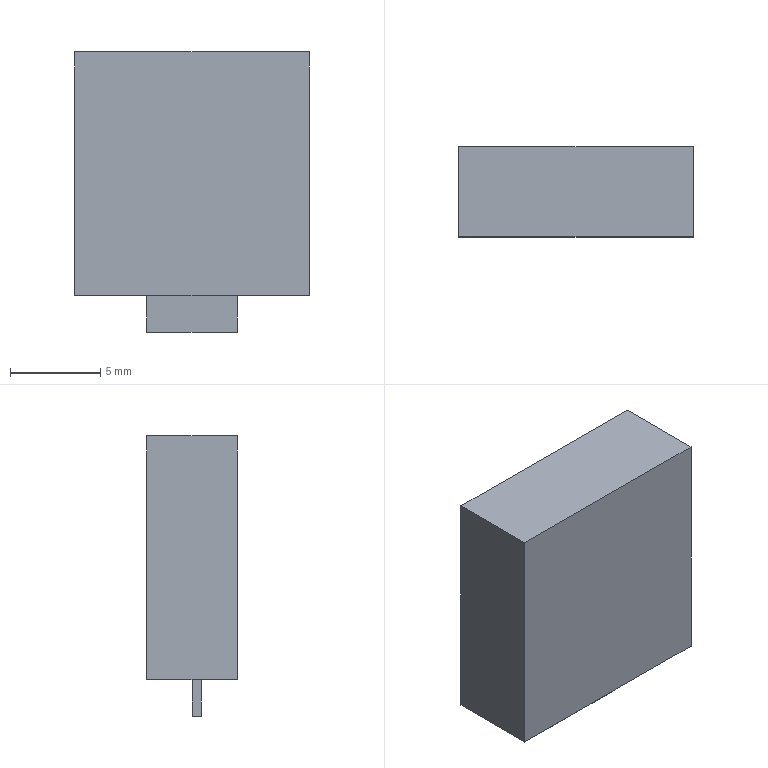Part | STEP file | 0245_028_FPCN14 | 1 solid | 11 faces | box 13 x 5 x 15.5 mm | volume 882.5 mm3 | plane 11
STEP:
#1=CARTESIAN_POINT('',(0.,0.,0.));
#2=DIRECTION('',(0.,0.,1.));
#3=DIRECTION('',(1.,0.,0.));
#4=AXIS2_PLACEMENT_3D('',#1,#2,#3);
#5=CARTESIAN_POINT('',(-6.5,5.,0.));
#6=VERTEX_POINT('',#5);
#7=CARTESIAN_POINT('',(-6.5,0.,0.));
#8=VERTEX_POINT('',#7);
#9=CARTESIAN_POINT('',(-6.5,0.,0.));
#10=DIRECTION('',(0.,-1.,0.));
#11=VECTOR('',#10,1.);
#12=LINE('',#9,#11);
#13=CARTESIAN_POINT('',(-6.5,5.,0.));
#14=DIRECTION('',(0.,0.,-1.));
#15=DIRECTION('',(-1.,0.,0.));
#16=AXIS2_PLACEMENT_3D('',#13,#14,#15);
#17=PLANE('',#16);
#18=CARTESIAN_POINT('',(0.,-5.));
#19=DIRECTION('',(0.,-1.));
#20=VECTOR('',#19,1.);
#21=LINE('',#18,#20);
#22=(GEOMETRIC_REPRESENTATION_CONTEXT(2)PARAMETRIC_REPRESENTATION_CONTEXT()REPRESENTATION_CONTEXT('',''));
#23=DEFINITIONAL_REPRESENTATION('',(#21),#22);
#24=PCURVE('',#17,#23);
#25=CARTESIAN_POINT('',(-6.5,0.,13.5));
#26=DIRECTION('',(1.,0.,0.));
#27=DIRECTION('',(0.,1.,0.));
#28=AXIS2_PLACEMENT_3D('',#25,#26,#27);
#29=PLANE('',#28);
#30=CARTESIAN_POINT('',(0.,-13.5));
#31=DIRECTION('',(-1.,0.));
#32=VECTOR('',#31,1.);
#33=LINE('',#30,#32);
#34=(GEOMETRIC_REPRESENTATION_CONTEXT(2)PARAMETRIC_REPRESENTATION_CONTEXT()REPRESENTATION_CONTEXT('',''));
#35=DEFINITIONAL_REPRESENTATION('',(#33),#34);
#36=PCURVE('',#29,#35);
#37=SURFACE_CURVE('',#12,(#24,#36),.PCURVE_S1.);
#38=EDGE_CURVE('',#6,#8,#37,.T.);
#39=ORIENTED_EDGE('',*,*,#38,.F.);
#40=CARTESIAN_POINT('',(6.5,5.,0.));
#41=VERTEX_POINT('',#40);
#42=CARTESIAN_POINT('',(-6.5,5.,0.));
#43=DIRECTION('',(-1.,0.,0.));
#44=VECTOR('',#43,1.);
#45=LINE('',#42,#44);
#46=CARTESIAN_POINT('',(0.,0.));
#47=DIRECTION('',(1.,0.));
#48=VECTOR('',#47,1.);
#49=LINE('',#46,#48);
#50=(GEOMETRIC_REPRESENTATION_CONTEXT(2)PARAMETRIC_REPRESENTATION_CONTEXT()REPRESENTATION_CONTEXT('',''));
#51=DEFINITIONAL_REPRESENTATION('',(#49),#50);
#52=PCURVE('',#17,#51);
#53=CARTESIAN_POINT('',(-6.5,5.,13.5));
#54=DIRECTION('',(0.,-1.,0.));
#55=DIRECTION('',(0.,0.,-1.));
#56=AXIS2_PLACEMENT_3D('',#53,#54,#55);
#57=PLANE('',#56);
#58=CARTESIAN_POINT('',(13.5,0.));
#59=DIRECTION('',(0.,-1.));
#60=VECTOR('',#59,1.);
#61=LINE('',#58,#60);
#62=(GEOMETRIC_REPRESENTATION_CONTEXT(2)PARAMETRIC_REPRESENTATION_CONTEXT()REPRESENTATION_CONTEXT('',''));
#63=DEFINITIONAL_REPRESENTATION('',(#61),#62);
#64=PCURVE('',#57,#63);
#65=SURFACE_CURVE('',#45,(#52,#64),.PCURVE_S1.);
#66=EDGE_CURVE('',#41,#6,#65,.T.);
#67=ORIENTED_EDGE('',*,*,#66,.F.);
#68=CARTESIAN_POINT('',(6.5,0.,0.));
#69=VERTEX_POINT('',#68);
#70=CARTESIAN_POINT('',(6.5,0.,0.));
#71=DIRECTION('',(0.,1.,0.));
#72=VECTOR('',#71,1.);
#73=LINE('',#70,#72);
#74=CARTESIAN_POINT('',(-13.,-5.));
#75=DIRECTION('',(0.,1.));
#76=VECTOR('',#75,1.);
#77=LINE('',#74,#76);
#78=(GEOMETRIC_REPRESENTATION_CONTEXT(2)PARAMETRIC_REPRESENTATION_CONTEXT()REPRESENTATION_CONTEXT('',''));
#79=DEFINITIONAL_REPRESENTATION('',(#77),#78);
#80=PCURVE('',#17,#79);
#81=CARTESIAN_POINT('',(6.5,0.,13.5));
#82=DIRECTION('',(-1.,0.,0.));
#83=DIRECTION('',(0.,-1.,0.));
#84=AXIS2_PLACEMENT_3D('',#81,#82,#83);
#85=PLANE('',#84);
#86=CARTESIAN_POINT('',(0.,-13.5));
#87=DIRECTION('',(-1.,0.));
#88=VECTOR('',#87,1.);
#89=LINE('',#86,#88);
#90=(GEOMETRIC_REPRESENTATION_CONTEXT(2)PARAMETRIC_REPRESENTATION_CONTEXT()REPRESENTATION_CONTEXT('',''));
#91=DEFINITIONAL_REPRESENTATION('',(#89),#90);
#92=PCURVE('',#85,#91);
#93=SURFACE_CURVE('',#73,(#80,#92),.PCURVE_S1.);
#94=EDGE_CURVE('',#69,#41,#93,.T.);
#95=ORIENTED_EDGE('',*,*,#94,.F.);
#96=CARTESIAN_POINT('',(-6.5,0.,0.));
#97=DIRECTION('',(1.,0.,0.));
#98=VECTOR('',#97,1.);
#99=LINE('',#96,#98);
#100=CARTESIAN_POINT('',(0.,-5.));
#101=DIRECTION('',(-1.,0.));
#102=VECTOR('',#101,1.);
#103=LINE('',#100,#102);
#104=(GEOMETRIC_REPRESENTATION_CONTEXT(2)PARAMETRIC_REPRESENTATION_CONTEXT()REPRESENTATION_CONTEXT('',''));
#105=DEFINITIONAL_REPRESENTATION('',(#103),#104);
#106=PCURVE('',#17,#105);
#107=CARTESIAN_POINT('',(-6.5,0.,13.5));
#108=DIRECTION('',(0.,1.,0.));
#109=DIRECTION('',(-1.,0.,0.));
#110=AXIS2_PLACEMENT_3D('',#107,#108,#109);
#111=PLANE('',#110);
#112=CARTESIAN_POINT('',(0.,-13.5));
#113=DIRECTION('',(-1.,0.));
#114=VECTOR('',#113,1.);
#115=LINE('',#112,#114);
#116=(GEOMETRIC_REPRESENTATION_CONTEXT(2)PARAMETRIC_REPRESENTATION_CONTEXT()REPRESENTATION_CONTEXT('',''));
#117=DEFINITIONAL_REPRESENTATION('',(#115),#116);
#118=PCURVE('',#111,#117);
#119=SURFACE_CURVE('',#99,(#106,#118),.PCURVE_S1.);
#120=EDGE_CURVE('',#8,#69,#119,.T.);
#121=ORIENTED_EDGE('',*,*,#120,.F.);
#122=EDGE_LOOP('',(#39,#67,#95,#121));
#123=FACE_BOUND('',#122,.T.);
#124=CARTESIAN_POINT('',(2.5,2.,0.));
#125=VERTEX_POINT('',#124);
#126=CARTESIAN_POINT('',(-2.5,2.,0.));
#127=VERTEX_POINT('',#126);
#128=CARTESIAN_POINT('',(2.5,2.,0.));
#129=DIRECTION('',(-1.,0.,0.));
#130=VECTOR('',#129,1.);
#131=LINE('',#128,#130);
#132=CARTESIAN_POINT('',(-9.,-3.));
#133=DIRECTION('',(1.,0.));
#134=VECTOR('',#133,1.);
#135=LINE('',#132,#134);
#136=(GEOMETRIC_REPRESENTATION_CONTEXT(2)PARAMETRIC_REPRESENTATION_CONTEXT()REPRESENTATION_CONTEXT('',''));
#137=DEFINITIONAL_REPRESENTATION('',(#135),#136);
#138=PCURVE('',#17,#137);
#139=CARTESIAN_POINT('',(2.5,2.,-2.));
#140=DIRECTION('',(0.,1.,0.));
#141=DIRECTION('',(0.,0.,1.));
#142=AXIS2_PLACEMENT_3D('',#139,#140,#141);
#143=PLANE('',#142);
#144=CARTESIAN_POINT('',(2.,0.));
#145=DIRECTION('',(0.,-1.));
#146=VECTOR('',#145,1.);
#147=LINE('',#144,#146);
#148=(GEOMETRIC_REPRESENTATION_CONTEXT(2)PARAMETRIC_REPRESENTATION_CONTEXT()REPRESENTATION_CONTEXT('',''));
#149=DEFINITIONAL_REPRESENTATION('',(#147),#148);
#150=PCURVE('',#143,#149);
#151=SURFACE_CURVE('',#131,(#138,#150),.PCURVE_S1.);
#152=EDGE_CURVE('',#125,#127,#151,.T.);
#153=ORIENTED_EDGE('',*,*,#152,.F.);
#154=CARTESIAN_POINT('',(2.5,2.5,0.));
#155=VERTEX_POINT('',#154);
#156=CARTESIAN_POINT('',(2.5,2.5,0.));
#157=DIRECTION('',(0.,-1.,0.));
#158=VECTOR('',#157,1.);
#159=LINE('',#156,#158);
#160=CARTESIAN_POINT('',(-9.,-2.5));
#161=DIRECTION('',(0.,-1.));
#162=VECTOR('',#161,1.);
#163=LINE('',#160,#162);
#164=(GEOMETRIC_REPRESENTATION_CONTEXT(2)PARAMETRIC_REPRESENTATION_CONTEXT()REPRESENTATION_CONTEXT('',''));
#165=DEFINITIONAL_REPRESENTATION('',(#163),#164);
#166=PCURVE('',#17,#165);
#167=CARTESIAN_POINT('',(2.5,2.5,-2.));
#168=DIRECTION('',(-1.,0.,0.));
#169=DIRECTION('',(0.,0.,1.));
#170=AXIS2_PLACEMENT_3D('',#167,#168,#169);
#171=PLANE('',#170);
#172=CARTESIAN_POINT('',(2.,0.));
#173=DIRECTION('',(0.,-1.));
#174=VECTOR('',#173,1.);
#175=LINE('',#172,#174);
#176=(GEOMETRIC_REPRESENTATION_CONTEXT(2)PARAMETRIC_REPRESENTATION_CONTEXT()REPRESENTATION_CONTEXT('',''));
#177=DEFINITIONAL_REPRESENTATION('',(#175),#176);
#178=PCURVE('',#171,#177);
#179=SURFACE_CURVE('',#159,(#166,#178),.PCURVE_S1.);
#180=EDGE_CURVE('',#155,#125,#179,.T.);
#181=ORIENTED_EDGE('',*,*,#180,.F.);
#182=CARTESIAN_POINT('',(-2.5,2.5,0.));
#183=VERTEX_POINT('',#182);
#184=CARTESIAN_POINT('',(2.5,2.5,0.));
#185=DIRECTION('',(1.,0.,0.));
#186=VECTOR('',#185,1.);
#187=LINE('',#184,#186);
#188=CARTESIAN_POINT('',(-9.,-2.5));
#189=DIRECTION('',(-1.,0.));
#190=VECTOR('',#189,1.);
#191=LINE('',#188,#190);
#192=(GEOMETRIC_REPRESENTATION_CONTEXT(2)PARAMETRIC_REPRESENTATION_CONTEXT()REPRESENTATION_CONTEXT('',''));
#193=DEFINITIONAL_REPRESENTATION('',(#191),#192);
#194=PCURVE('',#17,#193);
#195=CARTESIAN_POINT('',(2.5,2.5,-2.));
#196=DIRECTION('',(0.,-1.,0.));
#197=DIRECTION('',(0.,0.,-1.));
#198=AXIS2_PLACEMENT_3D('',#195,#196,#197);
#199=PLANE('',#198);
#200=CARTESIAN_POINT('',(-2.,0.));
#201=DIRECTION('',(0.,1.));
#202=VECTOR('',#201,1.);
#203=LINE('',#200,#202);
#204=(GEOMETRIC_REPRESENTATION_CONTEXT(2)PARAMETRIC_REPRESENTATION_CONTEXT()REPRESENTATION_CONTEXT('',''));
#205=DEFINITIONAL_REPRESENTATION('',(#203),#204);
#206=PCURVE('',#199,#205);
#207=SURFACE_CURVE('',#187,(#194,#206),.PCURVE_S1.);
#208=EDGE_CURVE('',#183,#155,#207,.T.);
#209=ORIENTED_EDGE('',*,*,#208,.F.);
#210=CARTESIAN_POINT('',(-2.5,2.5,0.));
#211=DIRECTION('',(0.,1.,0.));
#212=VECTOR('',#211,1.);
#213=LINE('',#210,#212);
#214=CARTESIAN_POINT('',(-4.,-2.5));
#215=DIRECTION('',(0.,1.));
#216=VECTOR('',#215,1.);
#217=LINE('',#214,#216);
#218=(GEOMETRIC_REPRESENTATION_CONTEXT(2)PARAMETRIC_REPRESENTATION_CONTEXT()REPRESENTATION_CONTEXT('',''));
#219=DEFINITIONAL_REPRESENTATION('',(#217),#218);
#220=PCURVE('',#17,#219);
#221=CARTESIAN_POINT('',(-2.5,2.5,-2.));
#222=DIRECTION('',(1.,0.,0.));
#223=DIRECTION('',(0.,0.,-1.));
#224=AXIS2_PLACEMENT_3D('',#221,#222,#223);
#225=PLANE('',#224);
#226=CARTESIAN_POINT('',(-2.,0.));
#227=DIRECTION('',(0.,1.));
#228=VECTOR('',#227,1.);
#229=LINE('',#226,#228);
#230=(GEOMETRIC_REPRESENTATION_CONTEXT(2)PARAMETRIC_REPRESENTATION_CONTEXT()REPRESENTATION_CONTEXT('',''));
#231=DEFINITIONAL_REPRESENTATION('',(#229),#230);
#232=PCURVE('',#225,#231);
#233=SURFACE_CURVE('',#213,(#220,#232),.PCURVE_S1.);
#234=EDGE_CURVE('',#127,#183,#233,.T.);
#235=ORIENTED_EDGE('',*,*,#234,.F.);
#236=EDGE_LOOP('',(#153,#181,#209,#235));
#237=FACE_BOUND('',#236,.T.);
#238=ADVANCED_FACE('',(#123,#237),#17,.T.);
#239=ORIENTED_EDGE('',*,*,#38,.T.);
#240=CARTESIAN_POINT('',(-6.5,0.,13.5));
#241=VERTEX_POINT('',#240);
#242=CARTESIAN_POINT('',(-6.5,0.,13.5));
#243=DIRECTION('',(0.,0.,-1.));
#244=VECTOR('',#243,1.);
#245=LINE('',#242,#244);
#246=CARTESIAN_POINT('',(0.,0.));
#247=DIRECTION('',(0.,-1.));
#248=VECTOR('',#247,1.);
#249=LINE('',#246,#248);
#250=(GEOMETRIC_REPRESENTATION_CONTEXT(2)PARAMETRIC_REPRESENTATION_CONTEXT()REPRESENTATION_CONTEXT('',''));
#251=DEFINITIONAL_REPRESENTATION('',(#249),#250);
#252=PCURVE('',#29,#251);
#253=CARTESIAN_POINT('',(0.,0.));
#254=DIRECTION('',(0.,-1.));
#255=VECTOR('',#254,1.);
#256=LINE('',#253,#255);
#257=(GEOMETRIC_REPRESENTATION_CONTEXT(2)PARAMETRIC_REPRESENTATION_CONTEXT()REPRESENTATION_CONTEXT('',''));
#258=DEFINITIONAL_REPRESENTATION('',(#256),#257);
#259=PCURVE('',#111,#258);
#260=SURFACE_CURVE('',#245,(#252,#259),.PCURVE_S1.);
#261=EDGE_CURVE('',#241,#8,#260,.T.);
#262=ORIENTED_EDGE('',*,*,#261,.F.);
#263=CARTESIAN_POINT('',(-6.5,5.,13.5));
#264=VERTEX_POINT('',#263);
#265=CARTESIAN_POINT('',(-6.5,0.,13.5));
#266=DIRECTION('',(0.,-1.,0.));
#267=VECTOR('',#266,1.);
#268=LINE('',#265,#267);
#269=CARTESIAN_POINT('',(0.,0.));
#270=DIRECTION('',(-1.,0.));
#271=VECTOR('',#270,1.);
#272=LINE('',#269,#271);
#273=(GEOMETRIC_REPRESENTATION_CONTEXT(2)PARAMETRIC_REPRESENTATION_CONTEXT()REPRESENTATION_CONTEXT('',''));
#274=DEFINITIONAL_REPRESENTATION('',(#272),#273);
#275=PCURVE('',#29,#274);
#276=CARTESIAN_POINT('',(-6.5,5.,13.5));
#277=DIRECTION('',(0.,0.,-1.));
#278=DIRECTION('',(-1.,0.,0.));
#279=AXIS2_PLACEMENT_3D('',#276,#277,#278);
#280=PLANE('',#279);
#281=CARTESIAN_POINT('',(0.,-5.));
#282=DIRECTION('',(0.,-1.));
#283=VECTOR('',#282,1.);
#284=LINE('',#281,#283);
#285=(GEOMETRIC_REPRESENTATION_CONTEXT(2)PARAMETRIC_REPRESENTATION_CONTEXT()REPRESENTATION_CONTEXT('',''));
#286=DEFINITIONAL_REPRESENTATION('',(#284),#285);
#287=PCURVE('',#280,#286);
#288=SURFACE_CURVE('',#268,(#275,#287),.PCURVE_S1.);
#289=EDGE_CURVE('',#264,#241,#288,.T.);
#290=ORIENTED_EDGE('',*,*,#289,.F.);
#291=CARTESIAN_POINT('',(-6.5,5.,13.5));
#292=DIRECTION('',(0.,0.,-1.));
#293=VECTOR('',#292,1.);
#294=LINE('',#291,#293);
#295=CARTESIAN_POINT('',(5.,0.));
#296=DIRECTION('',(0.,-1.));
#297=VECTOR('',#296,1.);
#298=LINE('',#295,#297);
#299=(GEOMETRIC_REPRESENTATION_CONTEXT(2)PARAMETRIC_REPRESENTATION_CONTEXT()REPRESENTATION_CONTEXT('',''));
#300=DEFINITIONAL_REPRESENTATION('',(#298),#299);
#301=PCURVE('',#29,#300);
#302=CARTESIAN_POINT('',(0.,0.));
#303=DIRECTION('',(1.,0.));
#304=VECTOR('',#303,1.);
#305=LINE('',#302,#304);
#306=(GEOMETRIC_REPRESENTATION_CONTEXT(2)PARAMETRIC_REPRESENTATION_CONTEXT()REPRESENTATION_CONTEXT('',''));
#307=DEFINITIONAL_REPRESENTATION('',(#305),#306);
#308=PCURVE('',#57,#307);
#309=SURFACE_CURVE('',#294,(#301,#308),.PCURVE_S1.);
#310=EDGE_CURVE('',#264,#6,#309,.T.);
#311=ORIENTED_EDGE('',*,*,#310,.T.);
#312=EDGE_LOOP('',(#239,#262,#290,#311));
#313=FACE_BOUND('',#312,.T.);
#314=ADVANCED_FACE('',(#313),#29,.F.);
#315=ORIENTED_EDGE('',*,*,#120,.T.);
#316=CARTESIAN_POINT('',(6.5,0.,13.5));
#317=VERTEX_POINT('',#316);
#318=CARTESIAN_POINT('',(6.5,0.,13.5));
#319=DIRECTION('',(0.,0.,-1.));
#320=VECTOR('',#319,1.);
#321=LINE('',#318,#320);
#322=CARTESIAN_POINT('',(-13.,0.));
#323=DIRECTION('',(0.,-1.));
#324=VECTOR('',#323,1.);
#325=LINE('',#322,#324);
#326=(GEOMETRIC_REPRESENTATION_CONTEXT(2)PARAMETRIC_REPRESENTATION_CONTEXT()REPRESENTATION_CONTEXT('',''));
#327=DEFINITIONAL_REPRESENTATION('',(#325),#326);
#328=PCURVE('',#111,#327);
#329=CARTESIAN_POINT('',(0.,0.));
#330=DIRECTION('',(0.,-1.));
#331=VECTOR('',#330,1.);
#332=LINE('',#329,#331);
#333=(GEOMETRIC_REPRESENTATION_CONTEXT(2)PARAMETRIC_REPRESENTATION_CONTEXT()REPRESENTATION_CONTEXT('',''));
#334=DEFINITIONAL_REPRESENTATION('',(#332),#333);
#335=PCURVE('',#85,#334);
#336=SURFACE_CURVE('',#321,(#328,#335),.PCURVE_S1.);
#337=EDGE_CURVE('',#317,#69,#336,.T.);
#338=ORIENTED_EDGE('',*,*,#337,.F.);
#339=CARTESIAN_POINT('',(-6.5,0.,13.5));
#340=DIRECTION('',(1.,0.,0.));
#341=VECTOR('',#340,1.);
#342=LINE('',#339,#341);
#343=CARTESIAN_POINT('',(0.,0.));
#344=DIRECTION('',(-1.,0.));
#345=VECTOR('',#344,1.);
#346=LINE('',#343,#345);
#347=(GEOMETRIC_REPRESENTATION_CONTEXT(2)PARAMETRIC_REPRESENTATION_CONTEXT()REPRESENTATION_CONTEXT('',''));
#348=DEFINITIONAL_REPRESENTATION('',(#346),#347);
#349=PCURVE('',#111,#348);
#350=CARTESIAN_POINT('',(0.,-5.));
#351=DIRECTION('',(-1.,0.));
#352=VECTOR('',#351,1.);
#353=LINE('',#350,#352);
#354=(GEOMETRIC_REPRESENTATION_CONTEXT(2)PARAMETRIC_REPRESENTATION_CONTEXT()REPRESENTATION_CONTEXT('',''));
#355=DEFINITIONAL_REPRESENTATION('',(#353),#354);
#356=PCURVE('',#280,#355);
#357=SURFACE_CURVE('',#342,(#349,#356),.PCURVE_S1.);
#358=EDGE_CURVE('',#241,#317,#357,.T.);
#359=ORIENTED_EDGE('',*,*,#358,.F.);
#360=ORIENTED_EDGE('',*,*,#261,.T.);
#361=EDGE_LOOP('',(#315,#338,#359,#360));
#362=FACE_BOUND('',#361,.T.);
#363=ADVANCED_FACE('',(#362),#111,.F.);
#364=ORIENTED_EDGE('',*,*,#94,.T.);
#365=CARTESIAN_POINT('',(6.5,5.,13.5));
#366=VERTEX_POINT('',#365);
#367=CARTESIAN_POINT('',(6.5,5.,13.5));
#368=DIRECTION('',(0.,0.,-1.));
#369=VECTOR('',#368,1.);
#370=LINE('',#367,#369);
#371=CARTESIAN_POINT('',(-5.,0.));
#372=DIRECTION('',(0.,-1.));
#373=VECTOR('',#372,1.);
#374=LINE('',#371,#373);
#375=(GEOMETRIC_REPRESENTATION_CONTEXT(2)PARAMETRIC_REPRESENTATION_CONTEXT()REPRESENTATION_CONTEXT('',''));
#376=DEFINITIONAL_REPRESENTATION('',(#374),#375);
#377=PCURVE('',#85,#376);
#378=CARTESIAN_POINT('',(0.,13.));
#379=DIRECTION('',(1.,0.));
#380=VECTOR('',#379,1.);
#381=LINE('',#378,#380);
#382=(GEOMETRIC_REPRESENTATION_CONTEXT(2)PARAMETRIC_REPRESENTATION_CONTEXT()REPRESENTATION_CONTEXT('',''));
#383=DEFINITIONAL_REPRESENTATION('',(#381),#382);
#384=PCURVE('',#57,#383);
#385=SURFACE_CURVE('',#370,(#377,#384),.PCURVE_S1.);
#386=EDGE_CURVE('',#366,#41,#385,.T.);
#387=ORIENTED_EDGE('',*,*,#386,.F.);
#388=CARTESIAN_POINT('',(6.5,0.,13.5));
#389=DIRECTION('',(0.,1.,0.));
#390=VECTOR('',#389,1.);
#391=LINE('',#388,#390);
#392=CARTESIAN_POINT('',(0.,0.));
#393=DIRECTION('',(-1.,0.));
#394=VECTOR('',#393,1.);
#395=LINE('',#392,#394);
#396=(GEOMETRIC_REPRESENTATION_CONTEXT(2)PARAMETRIC_REPRESENTATION_CONTEXT()REPRESENTATION_CONTEXT('',''));
#397=DEFINITIONAL_REPRESENTATION('',(#395),#396);
#398=PCURVE('',#85,#397);
#399=CARTESIAN_POINT('',(-13.,-5.));
#400=DIRECTION('',(0.,1.));
#401=VECTOR('',#400,1.);
#402=LINE('',#399,#401);
#403=(GEOMETRIC_REPRESENTATION_CONTEXT(2)PARAMETRIC_REPRESENTATION_CONTEXT()REPRESENTATION_CONTEXT('',''));
#404=DEFINITIONAL_REPRESENTATION('',(#402),#403);
#405=PCURVE('',#280,#404);
#406=SURFACE_CURVE('',#391,(#398,#405),.PCURVE_S1.);
#407=EDGE_CURVE('',#317,#366,#406,.T.);
#408=ORIENTED_EDGE('',*,*,#407,.F.);
#409=ORIENTED_EDGE('',*,*,#337,.T.);
#410=EDGE_LOOP('',(#364,#387,#408,#409));
#411=FACE_BOUND('',#410,.T.);
#412=ADVANCED_FACE('',(#411),#85,.F.);
#413=ORIENTED_EDGE('',*,*,#66,.T.);
#414=ORIENTED_EDGE('',*,*,#310,.F.);
#415=CARTESIAN_POINT('',(-6.5,5.,13.5));
#416=DIRECTION('',(-1.,0.,0.));
#417=VECTOR('',#416,1.);
#418=LINE('',#415,#417);
#419=CARTESIAN_POINT('',(0.,0.));
#420=DIRECTION('',(0.,-1.));
#421=VECTOR('',#420,1.);
#422=LINE('',#419,#421);
#423=(GEOMETRIC_REPRESENTATION_CONTEXT(2)PARAMETRIC_REPRESENTATION_CONTEXT()REPRESENTATION_CONTEXT('',''));
#424=DEFINITIONAL_REPRESENTATION('',(#422),#423);
#425=PCURVE('',#57,#424);
#426=CARTESIAN_POINT('',(0.,0.));
#427=DIRECTION('',(1.,0.));
#428=VECTOR('',#427,1.);
#429=LINE('',#426,#428);
#430=(GEOMETRIC_REPRESENTATION_CONTEXT(2)PARAMETRIC_REPRESENTATION_CONTEXT()REPRESENTATION_CONTEXT('',''));
#431=DEFINITIONAL_REPRESENTATION('',(#429),#430);
#432=PCURVE('',#280,#431);
#433=SURFACE_CURVE('',#418,(#425,#432),.PCURVE_S1.);
#434=EDGE_CURVE('',#366,#264,#433,.T.);
#435=ORIENTED_EDGE('',*,*,#434,.F.);
#436=ORIENTED_EDGE('',*,*,#386,.T.);
#437=EDGE_LOOP('',(#413,#414,#435,#436));
#438=FACE_BOUND('',#437,.T.);
#439=ADVANCED_FACE('',(#438),#57,.F.);
#440=ORIENTED_EDGE('',*,*,#289,.T.);
#441=ORIENTED_EDGE('',*,*,#358,.T.);
#442=ORIENTED_EDGE('',*,*,#407,.T.);
#443=ORIENTED_EDGE('',*,*,#434,.T.);
#444=EDGE_LOOP('',(#440,#441,#442,#443));
#445=FACE_BOUND('',#444,.T.);
#446=ADVANCED_FACE('',(#445),#280,.F.);
#447=ORIENTED_EDGE('',*,*,#180,.T.);
#448=CARTESIAN_POINT('',(2.5,2.,-2.));
#449=VERTEX_POINT('',#448);
#450=CARTESIAN_POINT('',(2.5,2.,-2.));
#451=DIRECTION('',(0.,0.,1.));
#452=VECTOR('',#451,1.);
#453=LINE('',#450,#452);
#454=CARTESIAN_POINT('',(0.,-0.5));
#455=DIRECTION('',(1.,0.));
#456=VECTOR('',#455,1.);
#457=LINE('',#454,#456);
#458=(GEOMETRIC_REPRESENTATION_CONTEXT(2)PARAMETRIC_REPRESENTATION_CONTEXT()REPRESENTATION_CONTEXT('',''));
#459=DEFINITIONAL_REPRESENTATION('',(#457),#458);
#460=PCURVE('',#171,#459);
#461=CARTESIAN_POINT('',(0.,0.));
#462=DIRECTION('',(1.,0.));
#463=VECTOR('',#462,1.);
#464=LINE('',#461,#463);
#465=(GEOMETRIC_REPRESENTATION_CONTEXT(2)PARAMETRIC_REPRESENTATION_CONTEXT()REPRESENTATION_CONTEXT('',''));
#466=DEFINITIONAL_REPRESENTATION('',(#464),#465);
#467=PCURVE('',#143,#466);
#468=SURFACE_CURVE('',#453,(#460,#467),.PCURVE_S1.);
#469=EDGE_CURVE('',#449,#125,#468,.T.);
#470=ORIENTED_EDGE('',*,*,#469,.F.);
#471=CARTESIAN_POINT('',(2.5,2.5,-2.));
#472=VERTEX_POINT('',#471);
#473=CARTESIAN_POINT('',(2.5,2.5,-2.));
#474=DIRECTION('',(0.,-1.,0.));
#475=VECTOR('',#474,1.);
#476=LINE('',#473,#475);
#477=CARTESIAN_POINT('',(0.,0.));
#478=DIRECTION('',(0.,-1.));
#479=VECTOR('',#478,1.);
#480=LINE('',#477,#479);
#481=(GEOMETRIC_REPRESENTATION_CONTEXT(2)PARAMETRIC_REPRESENTATION_CONTEXT()REPRESENTATION_CONTEXT('',''));
#482=DEFINITIONAL_REPRESENTATION('',(#480),#481);
#483=PCURVE('',#171,#482);
#484=CARTESIAN_POINT('',(2.5,2.,-2.));
#485=DIRECTION('',(0.,0.,-1.));
#486=DIRECTION('',(-1.,0.,0.));
#487=AXIS2_PLACEMENT_3D('',#484,#485,#486);
#488=PLANE('',#487);
#489=CARTESIAN_POINT('',(0.,0.5));
#490=DIRECTION('',(0.,-1.));
#491=VECTOR('',#490,1.);
#492=LINE('',#489,#491);
#493=(GEOMETRIC_REPRESENTATION_CONTEXT(2)PARAMETRIC_REPRESENTATION_CONTEXT()REPRESENTATION_CONTEXT('',''));
#494=DEFINITIONAL_REPRESENTATION('',(#492),#493);
#495=PCURVE('',#488,#494);
#496=SURFACE_CURVE('',#476,(#483,#495),.PCURVE_S1.);
#497=EDGE_CURVE('',#472,#449,#496,.T.);
#498=ORIENTED_EDGE('',*,*,#497,.F.);
#499=CARTESIAN_POINT('',(2.5,2.5,-2.));
#500=DIRECTION('',(0.,0.,1.));
#501=VECTOR('',#500,1.);
#502=LINE('',#499,#501);
#503=CARTESIAN_POINT('',(0.,0.));
#504=DIRECTION('',(1.,0.));
#505=VECTOR('',#504,1.);
#506=LINE('',#503,#505);
#507=(GEOMETRIC_REPRESENTATION_CONTEXT(2)PARAMETRIC_REPRESENTATION_CONTEXT()REPRESENTATION_CONTEXT('',''));
#508=DEFINITIONAL_REPRESENTATION('',(#506),#507);
#509=PCURVE('',#171,#508);
#510=CARTESIAN_POINT('',(0.,0.));
#511=DIRECTION('',(-1.,0.));
#512=VECTOR('',#511,1.);
#513=LINE('',#510,#512);
#514=(GEOMETRIC_REPRESENTATION_CONTEXT(2)PARAMETRIC_REPRESENTATION_CONTEXT()REPRESENTATION_CONTEXT('',''));
#515=DEFINITIONAL_REPRESENTATION('',(#513),#514);
#516=PCURVE('',#199,#515);
#517=SURFACE_CURVE('',#502,(#509,#516),.PCURVE_S1.);
#518=EDGE_CURVE('',#472,#155,#517,.T.);
#519=ORIENTED_EDGE('',*,*,#518,.T.);
#520=EDGE_LOOP('',(#447,#470,#498,#519));
#521=FACE_BOUND('',#520,.T.);
#522=ADVANCED_FACE('',(#521),#171,.F.);
#523=ORIENTED_EDGE('',*,*,#152,.T.);
#524=CARTESIAN_POINT('',(-2.5,2.,-2.));
#525=VERTEX_POINT('',#524);
#526=CARTESIAN_POINT('',(-2.5,2.,-2.));
#527=DIRECTION('',(0.,0.,1.));
#528=VECTOR('',#527,1.);
#529=LINE('',#526,#528);
#530=CARTESIAN_POINT('',(0.,-5.));
#531=DIRECTION('',(1.,0.));
#532=VECTOR('',#531,1.);
#533=LINE('',#530,#532);
#534=(GEOMETRIC_REPRESENTATION_CONTEXT(2)PARAMETRIC_REPRESENTATION_CONTEXT()REPRESENTATION_CONTEXT('',''));
#535=DEFINITIONAL_REPRESENTATION('',(#533),#534);
#536=PCURVE('',#143,#535);
#537=CARTESIAN_POINT('',(0.,-0.5));
#538=DIRECTION('',(-1.,0.));
#539=VECTOR('',#538,1.);
#540=LINE('',#537,#539);
#541=(GEOMETRIC_REPRESENTATION_CONTEXT(2)PARAMETRIC_REPRESENTATION_CONTEXT()REPRESENTATION_CONTEXT('',''));
#542=DEFINITIONAL_REPRESENTATION('',(#540),#541);
#543=PCURVE('',#225,#542);
#544=SURFACE_CURVE('',#529,(#536,#543),.PCURVE_S1.);
#545=EDGE_CURVE('',#525,#127,#544,.T.);
#546=ORIENTED_EDGE('',*,*,#545,.F.);
#547=CARTESIAN_POINT('',(2.5,2.,-2.));
#548=DIRECTION('',(-1.,0.,0.));
#549=VECTOR('',#548,1.);
#550=LINE('',#547,#549);
#551=CARTESIAN_POINT('',(0.,0.));
#552=DIRECTION('',(0.,-1.));
#553=VECTOR('',#552,1.);
#554=LINE('',#551,#553);
#555=(GEOMETRIC_REPRESENTATION_CONTEXT(2)PARAMETRIC_REPRESENTATION_CONTEXT()REPRESENTATION_CONTEXT('',''));
#556=DEFINITIONAL_REPRESENTATION('',(#554),#555);
#557=PCURVE('',#143,#556);
#558=CARTESIAN_POINT('',(0.,0.));
#559=DIRECTION('',(1.,0.));
#560=VECTOR('',#559,1.);
#561=LINE('',#558,#560);
#562=(GEOMETRIC_REPRESENTATION_CONTEXT(2)PARAMETRIC_REPRESENTATION_CONTEXT()REPRESENTATION_CONTEXT('',''));
#563=DEFINITIONAL_REPRESENTATION('',(#561),#562);
#564=PCURVE('',#488,#563);
#565=SURFACE_CURVE('',#550,(#557,#564),.PCURVE_S1.);
#566=EDGE_CURVE('',#449,#525,#565,.T.);
#567=ORIENTED_EDGE('',*,*,#566,.F.);
#568=ORIENTED_EDGE('',*,*,#469,.T.);
#569=EDGE_LOOP('',(#523,#546,#567,#568));
#570=FACE_BOUND('',#569,.T.);
#571=ADVANCED_FACE('',(#570),#143,.F.);
#572=ORIENTED_EDGE('',*,*,#234,.T.);
#573=CARTESIAN_POINT('',(-2.5,2.5,-2.));
#574=VERTEX_POINT('',#573);
#575=CARTESIAN_POINT('',(-2.5,2.5,-2.));
#576=DIRECTION('',(0.,0.,1.));
#577=VECTOR('',#576,1.);
#578=LINE('',#575,#577);
#579=CARTESIAN_POINT('',(0.,0.));
#580=DIRECTION('',(-1.,0.));
#581=VECTOR('',#580,1.);
#582=LINE('',#579,#581);
#583=(GEOMETRIC_REPRESENTATION_CONTEXT(2)PARAMETRIC_REPRESENTATION_CONTEXT()REPRESENTATION_CONTEXT('',''));
#584=DEFINITIONAL_REPRESENTATION('',(#582),#583);
#585=PCURVE('',#225,#584);
#586=CARTESIAN_POINT('',(0.,-5.));
#587=DIRECTION('',(-1.,0.));
#588=VECTOR('',#587,1.);
#589=LINE('',#586,#588);
#590=(GEOMETRIC_REPRESENTATION_CONTEXT(2)PARAMETRIC_REPRESENTATION_CONTEXT()REPRESENTATION_CONTEXT('',''));
#591=DEFINITIONAL_REPRESENTATION('',(#589),#590);
#592=PCURVE('',#199,#591);
#593=SURFACE_CURVE('',#578,(#585,#592),.PCURVE_S1.);
#594=EDGE_CURVE('',#574,#183,#593,.T.);
#595=ORIENTED_EDGE('',*,*,#594,.F.);
#596=CARTESIAN_POINT('',(-2.5,2.5,-2.));
#597=DIRECTION('',(0.,1.,0.));
#598=VECTOR('',#597,1.);
#599=LINE('',#596,#598);
#600=CARTESIAN_POINT('',(0.,0.));
#601=DIRECTION('',(0.,1.));
#602=VECTOR('',#601,1.);
#603=LINE('',#600,#602);
#604=(GEOMETRIC_REPRESENTATION_CONTEXT(2)PARAMETRIC_REPRESENTATION_CONTEXT()REPRESENTATION_CONTEXT('',''));
#605=DEFINITIONAL_REPRESENTATION('',(#603),#604);
#606=PCURVE('',#225,#605);
#607=CARTESIAN_POINT('',(5.,0.5));
#608=DIRECTION('',(0.,1.));
#609=VECTOR('',#608,1.);
#610=LINE('',#607,#609);
#611=(GEOMETRIC_REPRESENTATION_CONTEXT(2)PARAMETRIC_REPRESENTATION_CONTEXT()REPRESENTATION_CONTEXT('',''));
#612=DEFINITIONAL_REPRESENTATION('',(#610),#611);
#613=PCURVE('',#488,#612);
#614=SURFACE_CURVE('',#599,(#606,#613),.PCURVE_S1.);
#615=EDGE_CURVE('',#525,#574,#614,.T.);
#616=ORIENTED_EDGE('',*,*,#615,.F.);
#617=ORIENTED_EDGE('',*,*,#545,.T.);
#618=EDGE_LOOP('',(#572,#595,#616,#617));
#619=FACE_BOUND('',#618,.T.);
#620=ADVANCED_FACE('',(#619),#225,.F.);
#621=ORIENTED_EDGE('',*,*,#208,.T.);
#622=ORIENTED_EDGE('',*,*,#518,.F.);
#623=CARTESIAN_POINT('',(2.5,2.5,-2.));
#624=DIRECTION('',(1.,0.,0.));
#625=VECTOR('',#624,1.);
#626=LINE('',#623,#625);
#627=CARTESIAN_POINT('',(0.,0.));
#628=DIRECTION('',(0.,1.));
#629=VECTOR('',#628,1.);
#630=LINE('',#627,#629);
#631=(GEOMETRIC_REPRESENTATION_CONTEXT(2)PARAMETRIC_REPRESENTATION_CONTEXT()REPRESENTATION_CONTEXT('',''));
#632=DEFINITIONAL_REPRESENTATION('',(#630),#631);
#633=PCURVE('',#199,#632);
#634=CARTESIAN_POINT('',(0.,0.5));
#635=DIRECTION('',(-1.,0.));
#636=VECTOR('',#635,1.);
#637=LINE('',#634,#636);
#638=(GEOMETRIC_REPRESENTATION_CONTEXT(2)PARAMETRIC_REPRESENTATION_CONTEXT()REPRESENTATION_CONTEXT('',''));
#639=DEFINITIONAL_REPRESENTATION('',(#637),#638);
#640=PCURVE('',#488,#639);
#641=SURFACE_CURVE('',#626,(#633,#640),.PCURVE_S1.);
#642=EDGE_CURVE('',#574,#472,#641,.T.);
#643=ORIENTED_EDGE('',*,*,#642,.F.);
#644=ORIENTED_EDGE('',*,*,#594,.T.);
#645=EDGE_LOOP('',(#621,#622,#643,#644));
#646=FACE_BOUND('',#645,.T.);
#647=ADVANCED_FACE('',(#646),#199,.F.);
#648=ORIENTED_EDGE('',*,*,#497,.T.);
#649=ORIENTED_EDGE('',*,*,#566,.T.);
#650=ORIENTED_EDGE('',*,*,#615,.T.);
#651=ORIENTED_EDGE('',*,*,#642,.T.);
#652=EDGE_LOOP('',(#648,#649,#650,#651));
#653=FACE_BOUND('',#652,.T.);
#654=ADVANCED_FACE('',(#653),#488,.T.);
#655=CLOSED_SHELL('',(#238,#314,#363,#412,#439,#446,#522,#571,#620,#647,#654));
#656=MANIFOLD_SOLID_BREP('',#655);
#657=(LENGTH_UNIT()NAMED_UNIT(*)SI_UNIT(.MILLI.,.METRE.));
#658=UNCERTAINTY_MEASURE_WITH_UNIT(LENGTH_MEASURE(0.0000001),#657,'','');
#659=(NAMED_UNIT(*)PLANE_ANGLE_UNIT()SI_UNIT($,.RADIAN.));
#660=(NAMED_UNIT(*)SI_UNIT($,.STERADIAN.)SOLID_ANGLE_UNIT());
#661=(GEOMETRIC_REPRESENTATION_CONTEXT(3)GLOBAL_UNCERTAINTY_ASSIGNED_CONTEXT((#658))GLOBAL_UNIT_ASSIGNED_CONTEXT((#657,#659,#660))REPRESENTATION_CONTEXT('',''));
#662=ADVANCED_BREP_SHAPE_REPRESENTATION('',(#4,#656),#661);